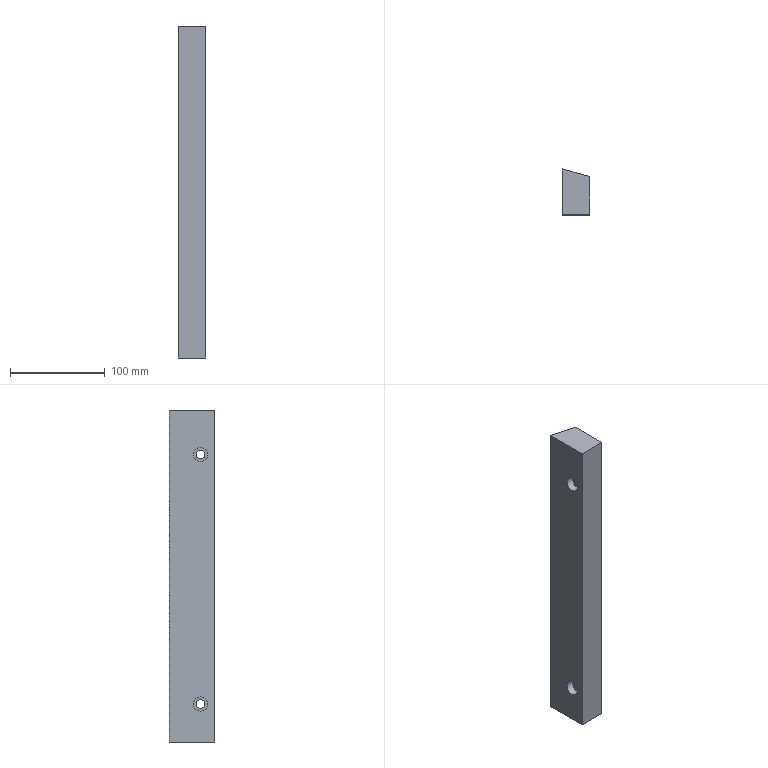Part | NX | features lower clamp support 2, MOVE_FACE 1 | 1 solid | 12 faces | box 29.5 x 47.905 x 350 mm | volume 448357 mm3 | plane 8 | cylinder 4 | commonest cylinder face diameters 9 x2 15 x2
STEP:
#1=CARTESIAN_POINT('',(-22.,-25.,-305.5));
#2=VERTEX_POINT('',#1);
#3=CARTESIAN_POINT('',(-22.,-25.,-310.));
#4=DIRECTION('',(-1.,0.,0.));
#5=DIRECTION('',(0.,0.,1.));
#6=AXIS2_PLACEMENT_3D('',#3,#4,#5);
#7=CIRCLE('',#6,4.5);
#8=EDGE_CURVE('',#2,#2,#7,.T.);
#9=ORIENTED_EDGE('',*,*,#8,.T.);
#10=EDGE_LOOP('',(#9));
#11=FACE_BOUND('',#10,.T.);
#12=CARTESIAN_POINT('',(0.,-25.,-305.5));
#13=VERTEX_POINT('',#12);
#14=CARTESIAN_POINT('',(0.,-25.,-310.));
#15=DIRECTION('',(-1.,0.,0.));
#16=DIRECTION('',(0.,0.,1.));
#17=AXIS2_PLACEMENT_3D('',#14,#15,#16);
#18=CIRCLE('',#17,4.5);
#19=EDGE_CURVE('',#13,#13,#18,.T.);
#20=ORIENTED_EDGE('',*,*,#19,.F.);
#21=EDGE_LOOP('',(#20));
#22=FACE_BOUND('',#21,.T.);
#23=CARTESIAN_POINT('',(-30.,-25.,-310.));
#24=DIRECTION('',(-1.,0.,0.));
#25=DIRECTION('',(0.,0.,1.));
#26=AXIS2_PLACEMENT_3D('',#23,#24,#25);
#27=CYLINDRICAL_SURFACE('',#26,4.5);
#28=ADVANCED_FACE('',(#11,#22),#27,.F.);
#29=CARTESIAN_POINT('',(-22.,-25.,-42.5));
#30=VERTEX_POINT('',#29);
#31=CARTESIAN_POINT('',(-22.,-25.,-47.));
#32=DIRECTION('',(-1.,0.,0.));
#33=DIRECTION('',(0.,0.,1.));
#34=AXIS2_PLACEMENT_3D('',#31,#32,#33);
#35=CIRCLE('',#34,4.5);
#36=EDGE_CURVE('',#30,#30,#35,.T.);
#37=ORIENTED_EDGE('',*,*,#36,.T.);
#38=EDGE_LOOP('',(#37));
#39=FACE_BOUND('',#38,.T.);
#40=CARTESIAN_POINT('',(0.,-25.,-42.5));
#41=VERTEX_POINT('',#40);
#42=CARTESIAN_POINT('',(0.,-25.,-47.));
#43=DIRECTION('',(-1.,0.,0.));
#44=DIRECTION('',(0.,0.,1.));
#45=AXIS2_PLACEMENT_3D('',#42,#43,#44);
#46=CIRCLE('',#45,4.5);
#47=EDGE_CURVE('',#41,#41,#46,.T.);
#48=ORIENTED_EDGE('',*,*,#47,.F.);
#49=EDGE_LOOP('',(#48));
#50=FACE_BOUND('',#49,.T.);
#51=CARTESIAN_POINT('',(-30.,-25.,-47.));
#52=DIRECTION('',(-1.,0.,0.));
#53=DIRECTION('',(0.,0.,1.));
#54=AXIS2_PLACEMENT_3D('',#51,#52,#53);
#55=CYLINDRICAL_SURFACE('',#54,4.5);
#56=ADVANCED_FACE('',(#39,#50),#55,.F.);
#57=CARTESIAN_POINT('',(-22.,-25.,-302.5));
#58=VERTEX_POINT('',#57);
#59=CARTESIAN_POINT('',(-22.,-25.,-310.));
#60=DIRECTION('',(-1.,0.,0.));
#61=DIRECTION('',(0.,0.,1.));
#62=AXIS2_PLACEMENT_3D('',#59,#60,#61);
#63=CIRCLE('',#62,7.5);
#64=EDGE_CURVE('',#58,#58,#63,.T.);
#65=ORIENTED_EDGE('',*,*,#64,.T.);
#66=EDGE_LOOP('',(#65));
#67=FACE_BOUND('',#66,.T.);
#68=ORIENTED_EDGE('',*,*,#8,.F.);
#69=EDGE_LOOP('',(#68));
#70=FACE_BOUND('',#69,.T.);
#71=CARTESIAN_POINT('',(-22.,-20.5,-310.));
#72=DIRECTION('',(1.,0.,0.));
#73=DIRECTION('',(0.,0.,-1.));
#74=AXIS2_PLACEMENT_3D('',#71,#72,#73);
#75=PLANE('',#74);
#76=ADVANCED_FACE('',(#67,#70),#75,.F.);
#77=CARTESIAN_POINT('',(-22.,-25.,-39.5));
#78=VERTEX_POINT('',#77);
#79=CARTESIAN_POINT('',(-22.,-25.,-47.));
#80=DIRECTION('',(-1.,0.,0.));
#81=DIRECTION('',(0.,0.,1.));
#82=AXIS2_PLACEMENT_3D('',#79,#80,#81);
#83=CIRCLE('',#82,7.5);
#84=EDGE_CURVE('',#78,#78,#83,.T.);
#85=ORIENTED_EDGE('',*,*,#84,.T.);
#86=EDGE_LOOP('',(#85));
#87=FACE_BOUND('',#86,.T.);
#88=ORIENTED_EDGE('',*,*,#36,.F.);
#89=EDGE_LOOP('',(#88));
#90=FACE_BOUND('',#89,.T.);
#91=CARTESIAN_POINT('',(-22.,-20.5,-47.));
#92=DIRECTION('',(1.,0.,0.));
#93=DIRECTION('',(0.,0.,-1.));
#94=AXIS2_PLACEMENT_3D('',#91,#92,#93);
#95=PLANE('',#94);
#96=ADVANCED_FACE('',(#87,#90),#95,.F.);
#97=CARTESIAN_POINT('',(0.,-40.,-350.));
#98=VERTEX_POINT('',#97);
#99=CARTESIAN_POINT('',(0.,0.,-350.));
#100=VERTEX_POINT('',#99);
#101=CARTESIAN_POINT('',(0.,-40.,-350.));
#102=DIRECTION('',(0.,1.,0.));
#103=VECTOR('',#102,1000.);
#104=LINE('',#101,#103);
#105=EDGE_CURVE('',#98,#100,#104,.T.);
#106=ORIENTED_EDGE('',*,*,#105,.T.);
#107=CARTESIAN_POINT('',(0.,0.,0.));
#108=VERTEX_POINT('',#107);
#109=CARTESIAN_POINT('',(0.,0.,-350.));
#110=DIRECTION('',(0.,0.,1.));
#111=VECTOR('',#110,1000.);
#112=LINE('',#109,#111);
#113=EDGE_CURVE('',#108,#100,#112,.F.);
#114=ORIENTED_EDGE('',*,*,#113,.F.);
#115=CARTESIAN_POINT('',(0.,-40.,0.));
#116=VERTEX_POINT('',#115);
#117=CARTESIAN_POINT('',(0.,-40.,0.));
#118=DIRECTION('',(0.,1.,0.));
#119=VECTOR('',#118,1000.);
#120=LINE('',#117,#119);
#121=EDGE_CURVE('',#116,#108,#120,.T.);
#122=ORIENTED_EDGE('',*,*,#121,.F.);
#123=CARTESIAN_POINT('',(0.,-40.,-350.));
#124=DIRECTION('',(0.,0.,1.));
#125=VECTOR('',#124,1000.);
#126=LINE('',#123,#125);
#127=EDGE_CURVE('',#98,#116,#126,.T.);
#128=ORIENTED_EDGE('',*,*,#127,.F.);
#129=EDGE_LOOP('',(#106,#114,#122,#128));
#130=FACE_BOUND('',#129,.T.);
#131=ORIENTED_EDGE('',*,*,#47,.T.);
#132=EDGE_LOOP('',(#131));
#133=FACE_BOUND('',#132,.T.);
#134=ORIENTED_EDGE('',*,*,#19,.T.);
#135=EDGE_LOOP('',(#134));
#136=FACE_BOUND('',#135,.T.);
#137=CARTESIAN_POINT('',(0.,-40.,-350.));
#138=DIRECTION('',(1.,0.,0.));
#139=DIRECTION('',(0.,0.,-1.));
#140=AXIS2_PLACEMENT_3D('',#137,#138,#139);
#141=PLANE('',#140);
#142=ADVANCED_FACE('',(#130,#133,#136),#141,.T.);
#143=CARTESIAN_POINT('',(-29.5,-25.,-302.5));
#144=VERTEX_POINT('',#143);
#145=CARTESIAN_POINT('',(-29.5,-25.,-310.));
#146=DIRECTION('',(-1.,0.,0.));
#147=DIRECTION('',(0.,0.,1.));
#148=AXIS2_PLACEMENT_3D('',#145,#146,#147);
#149=CIRCLE('',#148,7.5);
#150=EDGE_CURVE('',#144,#144,#149,.F.);
#151=ORIENTED_EDGE('',*,*,#150,.F.);
#152=EDGE_LOOP('',(#151));
#153=FACE_BOUND('',#152,.T.);
#154=ORIENTED_EDGE('',*,*,#64,.F.);
#155=EDGE_LOOP('',(#154));
#156=FACE_BOUND('',#155,.T.);
#157=CARTESIAN_POINT('',(-30.,-25.,-310.));
#158=DIRECTION('',(-1.,0.,0.));
#159=DIRECTION('',(0.,0.,1.));
#160=AXIS2_PLACEMENT_3D('',#157,#158,#159);
#161=CYLINDRICAL_SURFACE('',#160,7.5);
#162=ADVANCED_FACE('',(#153,#156),#161,.F.);
#163=CARTESIAN_POINT('',(-29.5,-25.,-39.5));
#164=VERTEX_POINT('',#163);
#165=CARTESIAN_POINT('',(-29.5,-25.,-47.));
#166=DIRECTION('',(-1.,0.,0.));
#167=DIRECTION('',(0.,0.,1.));
#168=AXIS2_PLACEMENT_3D('',#165,#166,#167);
#169=CIRCLE('',#168,7.5);
#170=EDGE_CURVE('',#164,#164,#169,.F.);
#171=ORIENTED_EDGE('',*,*,#170,.F.);
#172=EDGE_LOOP('',(#171));
#173=FACE_BOUND('',#172,.T.);
#174=ORIENTED_EDGE('',*,*,#84,.F.);
#175=EDGE_LOOP('',(#174));
#176=FACE_BOUND('',#175,.T.);
#177=CARTESIAN_POINT('',(-30.,-25.,-47.));
#178=DIRECTION('',(-1.,0.,0.));
#179=DIRECTION('',(0.,0.,1.));
#180=AXIS2_PLACEMENT_3D('',#177,#178,#179);
#181=CYLINDRICAL_SURFACE('',#180,7.5);
#182=ADVANCED_FACE('',(#173,#176),#181,.F.);
#183=CARTESIAN_POINT('',(-29.5,-40.,0.));
#184=VERTEX_POINT('',#183);
#185=CARTESIAN_POINT('',(-29.5,7.905,0.));
#186=VERTEX_POINT('',#185);
#187=CARTESIAN_POINT('',(-29.5,-40.,0.));
#188=DIRECTION('',(0.,1.,0.));
#189=VECTOR('',#188,1000.);
#190=LINE('',#187,#189);
#191=EDGE_CURVE('',#184,#186,#190,.T.);
#192=ORIENTED_EDGE('',*,*,#191,.F.);
#193=CARTESIAN_POINT('',(0.,-40.,0.));
#194=DIRECTION('',(1.,0.,0.));
#195=VECTOR('',#194,1000.);
#196=LINE('',#193,#195);
#197=EDGE_CURVE('',#116,#184,#196,.F.);
#198=ORIENTED_EDGE('',*,*,#197,.F.);
#199=ORIENTED_EDGE('',*,*,#121,.T.);
#200=CARTESIAN_POINT('',(0.,0.,0.));
#201=DIRECTION('',(-0.9659,0.2588,0.));
#202=VECTOR('',#201,1000.);
#203=LINE('',#200,#202);
#204=EDGE_CURVE('',#186,#108,#203,.F.);
#205=ORIENTED_EDGE('',*,*,#204,.F.);
#206=EDGE_LOOP('',(#192,#198,#199,#205));
#207=FACE_BOUND('',#206,.T.);
#208=CARTESIAN_POINT('',(0.,-40.,0.));
#209=DIRECTION('',(0.,0.,1.));
#210=DIRECTION('',(1.,0.,0.));
#211=AXIS2_PLACEMENT_3D('',#208,#209,#210);
#212=PLANE('',#211);
#213=ADVANCED_FACE('',(#207),#212,.T.);
#214=CARTESIAN_POINT('',(-29.5,7.905,-350.));
#215=VERTEX_POINT('',#214);
#216=CARTESIAN_POINT('',(0.,0.,-350.));
#217=DIRECTION('',(-0.9659,0.2588,0.));
#218=VECTOR('',#217,1000.);
#219=LINE('',#216,#218);
#220=EDGE_CURVE('',#100,#215,#219,.T.);
#221=ORIENTED_EDGE('',*,*,#220,.T.);
#222=CARTESIAN_POINT('',(-29.5,7.905,-350.));
#223=DIRECTION('',(0.,0.,-1.));
#224=VECTOR('',#223,1000.);
#225=LINE('',#222,#224);
#226=EDGE_CURVE('',#186,#215,#225,.T.);
#227=ORIENTED_EDGE('',*,*,#226,.F.);
#228=ORIENTED_EDGE('',*,*,#204,.T.);
#229=ORIENTED_EDGE('',*,*,#113,.T.);
#230=EDGE_LOOP('',(#221,#227,#228,#229));
#231=FACE_BOUND('',#230,.T.);
#232=CARTESIAN_POINT('',(0.,0.,-350.));
#233=DIRECTION('',(0.2588,0.9659,0.));
#234=DIRECTION('',(-0.9659,0.2588,0.));
#235=AXIS2_PLACEMENT_3D('',#232,#233,#234);
#236=PLANE('',#235);
#237=ADVANCED_FACE('',(#231),#236,.T.);
#238=CARTESIAN_POINT('',(-29.5,-40.,-350.));
#239=VERTEX_POINT('',#238);
#240=CARTESIAN_POINT('',(0.,-40.,-350.));
#241=DIRECTION('',(1.,0.,0.));
#242=VECTOR('',#241,1000.);
#243=LINE('',#240,#242);
#244=EDGE_CURVE('',#239,#98,#243,.T.);
#245=ORIENTED_EDGE('',*,*,#244,.F.);
#246=CARTESIAN_POINT('',(-29.5,-40.,-350.));
#247=DIRECTION('',(0.,1.,0.));
#248=VECTOR('',#247,1000.);
#249=LINE('',#246,#248);
#250=EDGE_CURVE('',#215,#239,#249,.F.);
#251=ORIENTED_EDGE('',*,*,#250,.F.);
#252=ORIENTED_EDGE('',*,*,#220,.F.);
#253=ORIENTED_EDGE('',*,*,#105,.F.);
#254=EDGE_LOOP('',(#245,#251,#252,#253));
#255=FACE_BOUND('',#254,.T.);
#256=CARTESIAN_POINT('',(0.,-40.,-350.));
#257=DIRECTION('',(0.,0.,1.));
#258=DIRECTION('',(1.,0.,0.));
#259=AXIS2_PLACEMENT_3D('',#256,#257,#258);
#260=PLANE('',#259);
#261=ADVANCED_FACE('',(#255),#260,.F.);
#262=ORIENTED_EDGE('',*,*,#244,.T.);
#263=ORIENTED_EDGE('',*,*,#127,.T.);
#264=ORIENTED_EDGE('',*,*,#197,.T.);
#265=CARTESIAN_POINT('',(-29.5,-40.,-350.));
#266=DIRECTION('',(0.,0.,1.));
#267=VECTOR('',#266,1000.);
#268=LINE('',#265,#267);
#269=EDGE_CURVE('',#239,#184,#268,.T.);
#270=ORIENTED_EDGE('',*,*,#269,.F.);
#271=EDGE_LOOP('',(#262,#263,#264,#270));
#272=FACE_BOUND('',#271,.T.);
#273=CARTESIAN_POINT('',(0.,-40.,-350.));
#274=DIRECTION('',(0.,-1.,0.));
#275=DIRECTION('',(1.,0.,0.));
#276=AXIS2_PLACEMENT_3D('',#273,#274,#275);
#277=PLANE('',#276);
#278=ADVANCED_FACE('',(#272),#277,.T.);
#279=ORIENTED_EDGE('',*,*,#250,.T.);
#280=ORIENTED_EDGE('',*,*,#269,.T.);
#281=ORIENTED_EDGE('',*,*,#191,.T.);
#282=ORIENTED_EDGE('',*,*,#226,.T.);
#283=EDGE_LOOP('',(#279,#280,#281,#282));
#284=FACE_BOUND('',#283,.T.);
#285=ORIENTED_EDGE('',*,*,#170,.T.);
#286=EDGE_LOOP('',(#285));
#287=FACE_BOUND('',#286,.T.);
#288=ORIENTED_EDGE('',*,*,#150,.T.);
#289=EDGE_LOOP('',(#288));
#290=FACE_BOUND('',#289,.T.);
#291=CARTESIAN_POINT('',(-29.5,-40.,-350.));
#292=DIRECTION('',(-1.,0.,0.));
#293=DIRECTION('',(0.,0.,1.));
#294=AXIS2_PLACEMENT_3D('',#291,#292,#293);
#295=PLANE('',#294);
#296=ADVANCED_FACE('',(#284,#287,#290),#295,.T.);
#297=CLOSED_SHELL('',(#28,#56,#76,#96,#142,#162,#182,#213,#237,#261,#278,#296));
#298=MANIFOLD_SOLID_BREP('',#297);
#299=(LENGTH_UNIT()NAMED_UNIT(*)SI_UNIT(.MILLI.,.METRE.));
#300=UNCERTAINTY_MEASURE_WITH_UNIT(LENGTH_MEASURE(0.00001),#299,'','');
#301=(NAMED_UNIT(*)PLANE_ANGLE_UNIT()SI_UNIT($,.RADIAN.));
#302=(NAMED_UNIT(*)SI_UNIT($,.STERADIAN.)SOLID_ANGLE_UNIT());
#303=(GEOMETRIC_REPRESENTATION_CONTEXT(3)GLOBAL_UNCERTAINTY_ASSIGNED_CONTEXT((#300))GLOBAL_UNIT_ASSIGNED_CONTEXT((#299,#301,#302))REPRESENTATION_CONTEXT('',''));
#304=ADVANCED_BREP_SHAPE_REPRESENTATION('',(#298),#303);